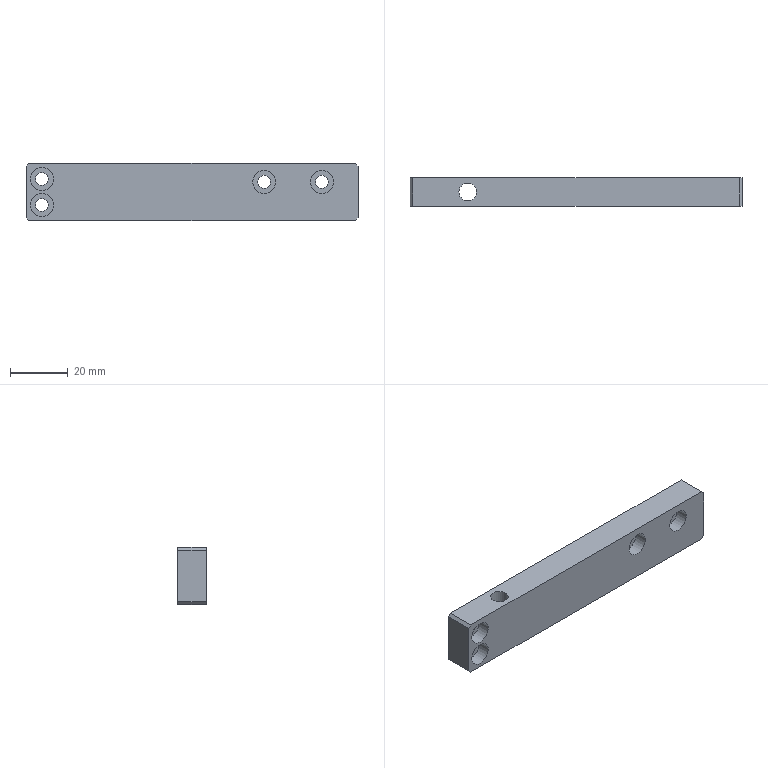CAM job | NX | 3+2 milling, drilling | part box 115 x 10 x 20 mm | stock box 120 x 12 x 25 mm
Tools:
number,name,description,diameter,corner_radius,flute_length,length,flutes
18,D2,平底铣刀-粗,2.0,0.0,50.0,75.0,2
4,D4,平底铣刀-粗,4.0,0.0,25.0,75.0,2
9,D10,平底铣刀-粗,10.0,0.0,35.0,75.0,2
19,D2-J,平底铣刀-精,2.0,0.0,50.0,75.0,2
18,D4-J,平底铣刀-精,4.0,0.0,50.0,75.0,2
10,D10-J,平底铣刀-精,10.0,0.0,35.0,75.0,2
1,D80R0.8飞刀,圆鼻刀-粗,80.0,0.8,50.0,75.0,2
1,D80R0.8飞刀-J,圆鼻刀-精,80.0,0.8,50.0,75.0,2
2,D6倒角刀,倒角刀,6.0,0.0,3.0,25.0,2
17,ZT3.8,钻头,3.8,0.0,35.0,50.0,2
11,ZT4.5,钻头,4.5,0.0,35.0,50.0,2
17,ZT6,钻头,6.0,0.0,35.0,50.0,2
Operations:
program,operation,operation_type,tool,method,geometry_group,spindle_rpm,surface_speed,feed_per_tooth,feed_cut,feed_plunge,cut_length_mm,path_length_mm,cut_time_min,machine_time_min
C,沉头孔打点-深0.8_2,Operation,D6倒角刀,NONE,W-C,8000.0,150.796,0.0312,500.0,90.0,1.8,43.6,0.0036,0.0078
C,沉头孔-钻孔0段_2,Operation,ZT6,NONE,W-C,2800.0,53.658,0.0357,200.0,90.0,24.803,89.605,0.124,0.1305
C,铣孔开粗D4_2,CylinderMilling,D4,NONE,W-C,8000.0,100.531,0.075,1200.0,100.0,123.599,165.099,0.103,0.1071
C,铣倒角_3,PlanarMilling,D6倒角刀,NONE,W-C,8000.0,150.796,0.0312,500.0,100.0,34.596,70.596,0.0692,0.0728
C,底壁铣精光侧面-中-选底面_COPY,VolumeBased25DMillingOperation,D4-J,侧刃精光-切深K-步距G,W-C,8000.0,100.531,0.0312,500.0,100.0,19.174,41.174,0.0383,0.0405
C,底壁铣精光侧面-中_COPY,VolumeBased25DMillingOperation,D4-J,侧刃精光-切深K-步距G,W-C,8000.0,100.531,0.0312,500.0,100.0,50.369,107.997,0.1007,0.1065
B,底壁铣飞面一刀开粗_COPY,VolumeBased25DMillingOperation,D80R0.8飞刀,分层开粗-切深K-步距G,W-B,5000.0,1256.637,0.3,3000.0,100.0,892.776,1584.735,0.2976,0.3668
B,底壁铣飞面一刀精光_COPY,VolumeBased25DMillingOperation,D80R0.8飞刀-J,侧刃精光-切深K-步距G,W-B,5000.0,1256.637,0.1,1000.0,100.0,222.998,258.998,0.223,0.2266
B,打点-深0.8,Operation,D6倒角刀,NONE,W-B,8000.0,150.796,0.0312,500.0,90.0,10.8,190.804,0.0216,0.0396
B,盲锥孔-精孔4.0预钻,Operation,ZT3.8,NONE,W-B,3000.0,35.814,0.0417,250.0,90.0,18.203,97.432,0.0728,0.0807
B,铣孔开粗D2_1,CylinderMilling,D2,NONE,W-B,8000.0,50.266,0.0375,600.0,100.0,195.538,308.538,0.3259,0.3372
B,钻倒角_1,Operation,D6倒角刀,METHOD,W-B,8000.0,150.796,0.0312,500.0,0.0,10.6,84.424,0.0212,0.0286
B,铣倒角_2,PlanarMilling,D6倒角刀,METHOD,W-B,8000.0,150.796,0.0312,500.0,100.0,69.412,337.287,0.1388,0.1656
B,铣孔精光D2_1,CylinderMilling,D2-J,精光步距切深关,W-B,8000.0,50.266,0.0125,200.0,100.0,116.877,229.877,0.5844,0.5957
A,顶面,FaceMilling,D80R0.8飞刀,侧刃精光-切深K-步距G,W-A,5000.0,1256.637,0.1,1000.0,100.0,209.0,245.0,0.209,0.2126
A,外形粗_2,VolumeBased25DMillingOperation,D10,METHOD,W-A,8000.0,251.327,0.3125,5000.0,80.0,4497.03,4545.63,0.8994,0.9043
A,沉头孔打点-深0.8,Operation,D6倒角刀,NONE,W-A,8000.0,150.796,0.0312,500.0,90.0,7.2,163.493,0.0144,0.03
A,沉头孔-钻孔0段,Operation,ZT4.5,NONE,W-A,2800.0,39.584,0.0357,200.0,90.0,57.408,263.909,0.287,0.3077
A,铣孔开粗D4_1,CylinderMilling,D4,NONE,W-A,8000.0,100.531,0.075,1200.0,100.0,851.827,1133.842,0.7099,0.7381
A,铣孔精光D4_1,CylinderMilling,D4,精光步距切深关,W-A,8000.0,100.531,0.0312,500.0,100.0,128.184,410.199,0.2564,0.2846
A,仅选体,SurfaceContour,D6倒角刀,METHOD,W-A,8000.0,150.796,0.1875,3000.0,100.0,284.959,320.76,0.095,0.0986
A,铣倒角_1,PlanarMilling,D6倒角刀,NONE,W-A,8000.0,150.796,0.0312,500.0,100.0,135.871,383.499,0.2717,0.2965
A,外形半精_2,VolumeBased25DMillingOperation,D10-J,METHOD,W-A,8000.0,251.327,0.0625,1000.0,100.0,304.031,363.231,0.304,0.31